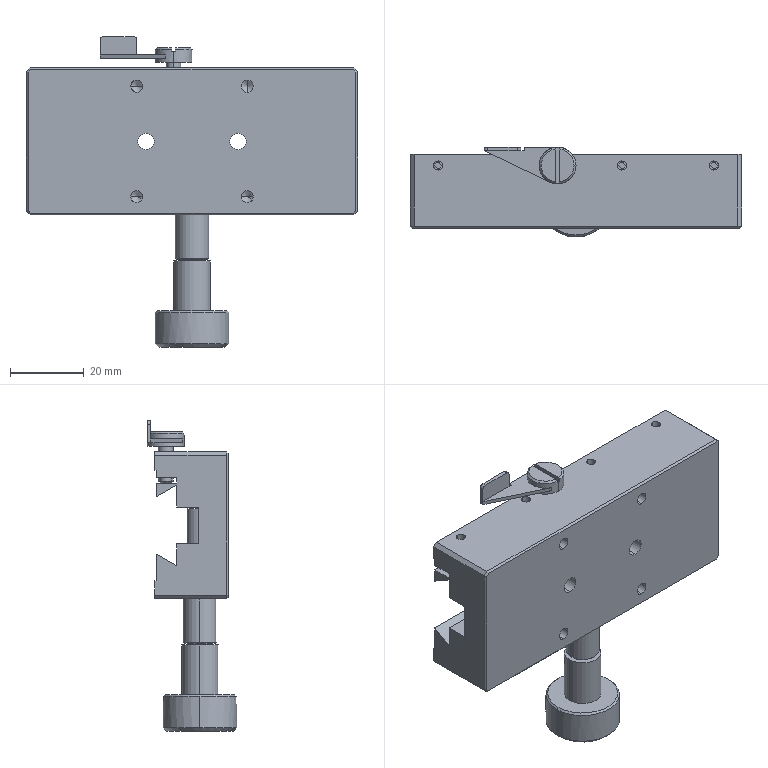Part | STEP file | Guide wheel mechanism revised.sldasm-Part-379 | 1 solid | 205 faces | box 90 x 24.3 x 84.5 mm | volume 59688 mm3 | plane 100 | cylinder 67 | cone 38 | commonest cylinder face diameters 2.5 x8 3 x8 3.3 x8 4 x6 4.5 x6 4.6 x4